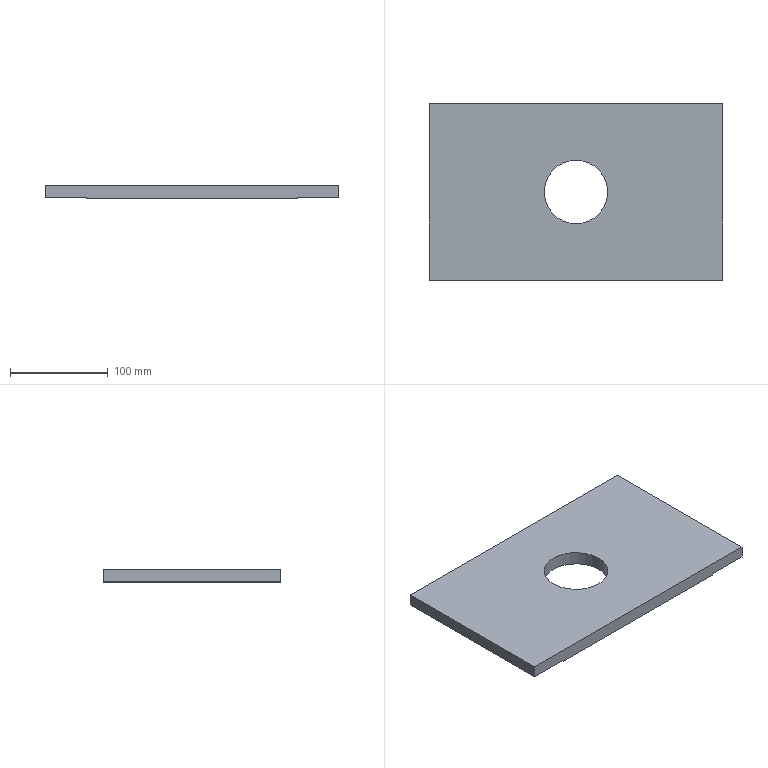Part | SolidWorks | features ICE 2, Extrusion 1 | 1 solid | 12 faces | box 300 x 180 x 14 mm | volume 686864 mm3 | plane 10 | cylinder 2 | commonest cylinder face diameters 65 x2
STEP:
#1=CARTESIAN_POINT('',(-32.5,0.,0.));
#2=VERTEX_POINT('',#1);
#3=CARTESIAN_POINT('',(32.5,0.,0.));
#4=VERTEX_POINT('',#3);
#5=CARTESIAN_POINT('',(0.,0.,0.));
#6=DIRECTION('',(0.,0.,1.));
#7=DIRECTION('',(-1.,0.,0.));
#8=AXIS2_PLACEMENT_3D('',#5,#6,#7);
#9=CIRCLE('',#8,32.5);
#10=EDGE_CURVE('',#2,#4,#9,.T.);
#11=ORIENTED_EDGE('',*,*,#10,.F.);
#12=CARTESIAN_POINT('',(-32.5,0.,14.));
#13=VERTEX_POINT('',#12);
#14=CARTESIAN_POINT('',(-32.5,0.,-0.001));
#15=DIRECTION('',(0.,0.,1.));
#16=VECTOR('',#15,1000.);
#17=LINE('',#14,#16);
#18=EDGE_CURVE('',#2,#13,#17,.T.);
#19=ORIENTED_EDGE('',*,*,#18,.T.);
#20=CARTESIAN_POINT('',(32.5,0.,14.));
#21=VERTEX_POINT('',#20);
#22=CARTESIAN_POINT('',(0.,0.,14.));
#23=DIRECTION('',(0.,0.,1.));
#24=DIRECTION('',(1.,0.,0.));
#25=AXIS2_PLACEMENT_3D('',#22,#23,#24);
#26=CIRCLE('',#25,32.5);
#27=EDGE_CURVE('',#13,#21,#26,.T.);
#28=ORIENTED_EDGE('',*,*,#27,.T.);
#29=CARTESIAN_POINT('',(32.5,0.,-0.001));
#30=DIRECTION('',(0.,0.,1.));
#31=VECTOR('',#30,1000.);
#32=LINE('',#29,#31);
#33=EDGE_CURVE('',#4,#21,#32,.T.);
#34=ORIENTED_EDGE('',*,*,#33,.F.);
#35=EDGE_LOOP('',(#11,#19,#28,#34));
#36=FACE_OUTER_BOUND('',#35,.T.);
#37=CARTESIAN_POINT('',(0.,0.,-0.001));
#38=DIRECTION('',(0.,0.,1.));
#39=DIRECTION('',(1.,0.,0.));
#40=AXIS2_PLACEMENT_3D('',#37,#38,#39);
#41=CYLINDRICAL_SURFACE('',#40,32.5);
#42=ADVANCED_FACE('',(#36),#41,.F.);
#43=CARTESIAN_POINT('',(-150.,-90.,1.5));
#44=VERTEX_POINT('',#43);
#45=CARTESIAN_POINT('',(-150.,90.,1.5));
#46=VERTEX_POINT('',#45);
#47=CARTESIAN_POINT('',(-150.,-90.,1.5));
#48=DIRECTION('',(0.,1.,0.));
#49=VECTOR('',#48,1000.);
#50=LINE('',#47,#49);
#51=EDGE_CURVE('',#44,#46,#50,.T.);
#52=ORIENTED_EDGE('',*,*,#51,.F.);
#53=CARTESIAN_POINT('',(-150.,-90.,14.));
#54=VERTEX_POINT('',#53);
#55=CARTESIAN_POINT('',(-150.,-90.,14.));
#56=DIRECTION('',(0.,0.,-1.));
#57=VECTOR('',#56,1000.);
#58=LINE('',#55,#57);
#59=EDGE_CURVE('',#54,#44,#58,.T.);
#60=ORIENTED_EDGE('',*,*,#59,.F.);
#61=CARTESIAN_POINT('',(-150.,90.,14.));
#62=VERTEX_POINT('',#61);
#63=CARTESIAN_POINT('',(-150.,-90.,14.));
#64=DIRECTION('',(0.,-1.,0.));
#65=VECTOR('',#64,1000.);
#66=LINE('',#63,#65);
#67=EDGE_CURVE('',#62,#54,#66,.T.);
#68=ORIENTED_EDGE('',*,*,#67,.F.);
#69=CARTESIAN_POINT('',(-150.,90.,14.));
#70=DIRECTION('',(0.,0.,-1.));
#71=VECTOR('',#70,1000.);
#72=LINE('',#69,#71);
#73=EDGE_CURVE('',#62,#46,#72,.T.);
#74=ORIENTED_EDGE('',*,*,#73,.T.);
#75=EDGE_LOOP('',(#52,#60,#68,#74));
#76=FACE_OUTER_BOUND('',#75,.T.);
#77=CARTESIAN_POINT('',(-150.,-90.,14.));
#78=DIRECTION('',(1.,0.,0.));
#79=DIRECTION('',(0.,0.,-1.));
#80=AXIS2_PLACEMENT_3D('',#77,#78,#79);
#81=PLANE('',#80);
#82=ADVANCED_FACE('',(#76),#81,.F.);
#83=CARTESIAN_POINT('',(150.,-90.,14.));
#84=VERTEX_POINT('',#83);
#85=CARTESIAN_POINT('',(150.,-90.,1.5));
#86=VERTEX_POINT('',#85);
#87=CARTESIAN_POINT('',(150.,-90.,14.));
#88=DIRECTION('',(0.,0.,-1.));
#89=VECTOR('',#88,1000.);
#90=LINE('',#87,#89);
#91=EDGE_CURVE('',#84,#86,#90,.T.);
#92=ORIENTED_EDGE('',*,*,#91,.T.);
#93=CARTESIAN_POINT('',(150.,90.,1.5));
#94=VERTEX_POINT('',#93);
#95=CARTESIAN_POINT('',(150.,-90.,1.5));
#96=DIRECTION('',(0.,-1.,0.));
#97=VECTOR('',#96,1000.);
#98=LINE('',#95,#97);
#99=EDGE_CURVE('',#94,#86,#98,.T.);
#100=ORIENTED_EDGE('',*,*,#99,.F.);
#101=CARTESIAN_POINT('',(150.,90.,14.));
#102=VERTEX_POINT('',#101);
#103=CARTESIAN_POINT('',(150.,90.,14.));
#104=DIRECTION('',(0.,0.,-1.));
#105=VECTOR('',#104,1000.);
#106=LINE('',#103,#105);
#107=EDGE_CURVE('',#102,#94,#106,.T.);
#108=ORIENTED_EDGE('',*,*,#107,.F.);
#109=CARTESIAN_POINT('',(150.,-90.,14.));
#110=DIRECTION('',(0.,1.,0.));
#111=VECTOR('',#110,1000.);
#112=LINE('',#109,#111);
#113=EDGE_CURVE('',#84,#102,#112,.T.);
#114=ORIENTED_EDGE('',*,*,#113,.F.);
#115=EDGE_LOOP('',(#92,#100,#108,#114));
#116=FACE_OUTER_BOUND('',#115,.T.);
#117=CARTESIAN_POINT('',(150.,-90.,14.));
#118=DIRECTION('',(-1.,0.,0.));
#119=DIRECTION('',(0.,0.,1.));
#120=AXIS2_PLACEMENT_3D('',#117,#118,#119);
#121=PLANE('',#120);
#122=ADVANCED_FACE('',(#116),#121,.F.);
#123=CARTESIAN_POINT('',(108.,90.,0.));
#124=VERTEX_POINT('',#123);
#125=CARTESIAN_POINT('',(-108.,90.,0.));
#126=VERTEX_POINT('',#125);
#127=CARTESIAN_POINT('',(-150.,90.,0.));
#128=DIRECTION('',(-1.,0.,0.));
#129=VECTOR('',#128,1000.);
#130=LINE('',#127,#129);
#131=EDGE_CURVE('',#124,#126,#130,.T.);
#132=ORIENTED_EDGE('',*,*,#131,.T.);
#133=CARTESIAN_POINT('',(-108.,90.,1.5));
#134=VERTEX_POINT('',#133);
#135=CARTESIAN_POINT('',(-108.,90.,1.5));
#136=DIRECTION('',(0.,0.,-1.));
#137=VECTOR('',#136,1000.);
#138=LINE('',#135,#137);
#139=EDGE_CURVE('',#134,#126,#138,.T.);
#140=ORIENTED_EDGE('',*,*,#139,.F.);
#141=CARTESIAN_POINT('',(-150.,90.,1.5));
#142=DIRECTION('',(1.,0.,0.));
#143=VECTOR('',#142,1000.);
#144=LINE('',#141,#143);
#145=EDGE_CURVE('',#46,#134,#144,.T.);
#146=ORIENTED_EDGE('',*,*,#145,.F.);
#147=ORIENTED_EDGE('',*,*,#73,.F.);
#148=CARTESIAN_POINT('',(-150.,90.,14.));
#149=DIRECTION('',(-1.,0.,0.));
#150=VECTOR('',#149,1000.);
#151=LINE('',#148,#150);
#152=EDGE_CURVE('',#102,#62,#151,.T.);
#153=ORIENTED_EDGE('',*,*,#152,.F.);
#154=ORIENTED_EDGE('',*,*,#107,.T.);
#155=CARTESIAN_POINT('',(108.,90.,1.5));
#156=VERTEX_POINT('',#155);
#157=CARTESIAN_POINT('',(150.,90.,1.5));
#158=DIRECTION('',(1.,0.,0.));
#159=VECTOR('',#158,1000.);
#160=LINE('',#157,#159);
#161=EDGE_CURVE('',#156,#94,#160,.T.);
#162=ORIENTED_EDGE('',*,*,#161,.F.);
#163=CARTESIAN_POINT('',(108.,90.,1.5));
#164=DIRECTION('',(0.,0.,-1.));
#165=VECTOR('',#164,1000.);
#166=LINE('',#163,#165);
#167=EDGE_CURVE('',#156,#124,#166,.T.);
#168=ORIENTED_EDGE('',*,*,#167,.T.);
#169=EDGE_LOOP('',(#132,#140,#146,#147,#153,#154,#162,#168));
#170=FACE_OUTER_BOUND('',#169,.T.);
#171=CARTESIAN_POINT('',(-150.,90.,14.));
#172=DIRECTION('',(0.,-1.,0.));
#173=DIRECTION('',(0.,0.,-1.));
#174=AXIS2_PLACEMENT_3D('',#171,#172,#173);
#175=PLANE('',#174);
#176=ADVANCED_FACE('',(#170),#175,.F.);
#177=CARTESIAN_POINT('',(-108.,-90.,1.5));
#178=VERTEX_POINT('',#177);
#179=CARTESIAN_POINT('',(-150.,-90.,1.5));
#180=DIRECTION('',(-1.,0.,0.));
#181=VECTOR('',#180,1000.);
#182=LINE('',#179,#181);
#183=EDGE_CURVE('',#178,#44,#182,.T.);
#184=ORIENTED_EDGE('',*,*,#183,.F.);
#185=CARTESIAN_POINT('',(-108.,-90.,0.));
#186=VERTEX_POINT('',#185);
#187=CARTESIAN_POINT('',(-108.,-90.,1.5));
#188=DIRECTION('',(0.,0.,-1.));
#189=VECTOR('',#188,1000.);
#190=LINE('',#187,#189);
#191=EDGE_CURVE('',#178,#186,#190,.T.);
#192=ORIENTED_EDGE('',*,*,#191,.T.);
#193=CARTESIAN_POINT('',(108.,-90.,0.));
#194=VERTEX_POINT('',#193);
#195=CARTESIAN_POINT('',(-150.,-90.,0.));
#196=DIRECTION('',(1.,0.,0.));
#197=VECTOR('',#196,1000.);
#198=LINE('',#195,#197);
#199=EDGE_CURVE('',#186,#194,#198,.T.);
#200=ORIENTED_EDGE('',*,*,#199,.T.);
#201=CARTESIAN_POINT('',(108.,-90.,1.5));
#202=VERTEX_POINT('',#201);
#203=CARTESIAN_POINT('',(108.,-90.,1.5));
#204=DIRECTION('',(0.,0.,-1.));
#205=VECTOR('',#204,1000.);
#206=LINE('',#203,#205);
#207=EDGE_CURVE('',#202,#194,#206,.T.);
#208=ORIENTED_EDGE('',*,*,#207,.F.);
#209=CARTESIAN_POINT('',(150.,-90.,1.5));
#210=DIRECTION('',(-1.,0.,0.));
#211=VECTOR('',#210,1000.);
#212=LINE('',#209,#211);
#213=EDGE_CURVE('',#86,#202,#212,.T.);
#214=ORIENTED_EDGE('',*,*,#213,.F.);
#215=ORIENTED_EDGE('',*,*,#91,.F.);
#216=CARTESIAN_POINT('',(-150.,-90.,14.));
#217=DIRECTION('',(1.,0.,0.));
#218=VECTOR('',#217,1000.);
#219=LINE('',#216,#218);
#220=EDGE_CURVE('',#54,#84,#219,.T.);
#221=ORIENTED_EDGE('',*,*,#220,.F.);
#222=ORIENTED_EDGE('',*,*,#59,.T.);
#223=EDGE_LOOP('',(#184,#192,#200,#208,#214,#215,#221,#222));
#224=FACE_OUTER_BOUND('',#223,.T.);
#225=CARTESIAN_POINT('',(-150.,-90.,14.));
#226=DIRECTION('',(0.,1.,0.));
#227=DIRECTION('',(0.,0.,1.));
#228=AXIS2_PLACEMENT_3D('',#225,#226,#227);
#229=PLANE('',#228);
#230=ADVANCED_FACE('',(#224),#229,.F.);
#231=CARTESIAN_POINT('',(0.,0.,14.));
#232=DIRECTION('',(0.,0.,1.));
#233=DIRECTION('',(1.,0.,0.));
#234=AXIS2_PLACEMENT_3D('',#231,#232,#233);
#235=CIRCLE('',#234,32.5);
#236=EDGE_CURVE('',#21,#13,#235,.T.);
#237=ORIENTED_EDGE('',*,*,#236,.F.);
#238=ORIENTED_EDGE('',*,*,#27,.F.);
#239=EDGE_LOOP('',(#237,#238));
#240=FACE_BOUND('',#239,.T.);
#241=ORIENTED_EDGE('',*,*,#113,.T.);
#242=ORIENTED_EDGE('',*,*,#152,.T.);
#243=ORIENTED_EDGE('',*,*,#67,.T.);
#244=ORIENTED_EDGE('',*,*,#220,.T.);
#245=EDGE_LOOP('',(#241,#242,#243,#244));
#246=FACE_OUTER_BOUND('',#245,.T.);
#247=CARTESIAN_POINT('',(0.,0.,14.));
#248=DIRECTION('',(0.,0.,-1.));
#249=DIRECTION('',(-1.,0.,0.));
#250=AXIS2_PLACEMENT_3D('',#247,#248,#249);
#251=PLANE('',#250);
#252=ADVANCED_FACE('',(#240,#246),#251,.F.);
#253=CARTESIAN_POINT('',(0.,0.,0.));
#254=DIRECTION('',(0.,0.,1.));
#255=DIRECTION('',(-1.,0.,0.));
#256=AXIS2_PLACEMENT_3D('',#253,#254,#255);
#257=CIRCLE('',#256,32.5);
#258=EDGE_CURVE('',#4,#2,#257,.T.);
#259=ORIENTED_EDGE('',*,*,#258,.T.);
#260=ORIENTED_EDGE('',*,*,#10,.T.);
#261=EDGE_LOOP('',(#259,#260));
#262=FACE_BOUND('',#261,.T.);
#263=CARTESIAN_POINT('',(-108.,-90.,0.));
#264=DIRECTION('',(0.,-1.,0.));
#265=VECTOR('',#264,1000.);
#266=LINE('',#263,#265);
#267=EDGE_CURVE('',#126,#186,#266,.T.);
#268=ORIENTED_EDGE('',*,*,#267,.F.);
#269=ORIENTED_EDGE('',*,*,#131,.F.);
#270=CARTESIAN_POINT('',(108.,-90.,0.));
#271=DIRECTION('',(0.,1.,0.));
#272=VECTOR('',#271,1000.);
#273=LINE('',#270,#272);
#274=EDGE_CURVE('',#194,#124,#273,.T.);
#275=ORIENTED_EDGE('',*,*,#274,.F.);
#276=ORIENTED_EDGE('',*,*,#199,.F.);
#277=EDGE_LOOP('',(#268,#269,#275,#276));
#278=FACE_OUTER_BOUND('',#277,.T.);
#279=CARTESIAN_POINT('',(0.,0.,0.));
#280=DIRECTION('',(0.,0.,-1.));
#281=DIRECTION('',(-1.,0.,0.));
#282=AXIS2_PLACEMENT_3D('',#279,#280,#281);
#283=PLANE('',#282);
#284=ADVANCED_FACE('',(#262,#278),#283,.T.);
#285=ORIENTED_EDGE('',*,*,#274,.T.);
#286=ORIENTED_EDGE('',*,*,#167,.F.);
#287=CARTESIAN_POINT('',(108.,-90.,1.5));
#288=DIRECTION('',(0.,1.,0.));
#289=VECTOR('',#288,1000.);
#290=LINE('',#287,#289);
#291=EDGE_CURVE('',#202,#156,#290,.T.);
#292=ORIENTED_EDGE('',*,*,#291,.F.);
#293=ORIENTED_EDGE('',*,*,#207,.T.);
#294=EDGE_LOOP('',(#285,#286,#292,#293));
#295=FACE_OUTER_BOUND('',#294,.T.);
#296=CARTESIAN_POINT('',(108.,-90.,1.5));
#297=DIRECTION('',(-1.,0.,0.));
#298=DIRECTION('',(0.,0.,1.));
#299=AXIS2_PLACEMENT_3D('',#296,#297,#298);
#300=PLANE('',#299);
#301=ADVANCED_FACE('',(#295),#300,.F.);
#302=ORIENTED_EDGE('',*,*,#99,.T.);
#303=ORIENTED_EDGE('',*,*,#213,.T.);
#304=ORIENTED_EDGE('',*,*,#291,.T.);
#305=ORIENTED_EDGE('',*,*,#161,.T.);
#306=EDGE_LOOP('',(#302,#303,#304,#305));
#307=FACE_OUTER_BOUND('',#306,.T.);
#308=CARTESIAN_POINT('',(0.,0.,1.5));
#309=DIRECTION('',(0.,0.,1.));
#310=DIRECTION('',(1.,0.,0.));
#311=AXIS2_PLACEMENT_3D('',#308,#309,#310);
#312=PLANE('',#311);
#313=ADVANCED_FACE('',(#307),#312,.F.);
#314=ORIENTED_EDGE('',*,*,#267,.T.);
#315=ORIENTED_EDGE('',*,*,#191,.F.);
#316=CARTESIAN_POINT('',(-108.,-90.,1.5));
#317=DIRECTION('',(0.,-1.,0.));
#318=VECTOR('',#317,1000.);
#319=LINE('',#316,#318);
#320=EDGE_CURVE('',#134,#178,#319,.T.);
#321=ORIENTED_EDGE('',*,*,#320,.F.);
#322=ORIENTED_EDGE('',*,*,#139,.T.);
#323=EDGE_LOOP('',(#314,#315,#321,#322));
#324=FACE_OUTER_BOUND('',#323,.T.);
#325=CARTESIAN_POINT('',(-108.,-90.,1.5));
#326=DIRECTION('',(1.,0.,0.));
#327=DIRECTION('',(0.,1.,0.));
#328=AXIS2_PLACEMENT_3D('',#325,#326,#327);
#329=PLANE('',#328);
#330=ADVANCED_FACE('',(#324),#329,.F.);
#331=ORIENTED_EDGE('',*,*,#51,.T.);
#332=ORIENTED_EDGE('',*,*,#145,.T.);
#333=ORIENTED_EDGE('',*,*,#320,.T.);
#334=ORIENTED_EDGE('',*,*,#183,.T.);
#335=EDGE_LOOP('',(#331,#332,#333,#334));
#336=FACE_OUTER_BOUND('',#335,.T.);
#337=CARTESIAN_POINT('',(0.,0.,1.5));
#338=DIRECTION('',(0.,0.,-1.));
#339=DIRECTION('',(-1.,0.,0.));
#340=AXIS2_PLACEMENT_3D('',#337,#338,#339);
#341=PLANE('',#340);
#342=ADVANCED_FACE('',(#336),#341,.T.);
#343=ORIENTED_EDGE('',*,*,#18,.F.);
#344=ORIENTED_EDGE('',*,*,#258,.F.);
#345=ORIENTED_EDGE('',*,*,#33,.T.);
#346=ORIENTED_EDGE('',*,*,#236,.T.);
#347=EDGE_LOOP('',(#343,#344,#345,#346));
#348=FACE_OUTER_BOUND('',#347,.T.);
#349=CARTESIAN_POINT('',(0.,0.,-0.001));
#350=DIRECTION('',(0.,0.,1.));
#351=DIRECTION('',(1.,0.,0.));
#352=AXIS2_PLACEMENT_3D('',#349,#350,#351);
#353=CYLINDRICAL_SURFACE('',#352,32.5);
#354=ADVANCED_FACE('',(#348),#353,.F.);
#355=CLOSED_SHELL('',(#42,#82,#122,#176,#230,#252,#284,#301,#313,#330,#342,#354));
#356=MANIFOLD_SOLID_BREP('',#355);
#357=CARTESIAN_POINT('',(0.,0.,0.));
#358=DIRECTION('',(0.,0.,1.));
#359=DIRECTION('',(1.,0.,0.));
#360=AXIS2_PLACEMENT_3D('',#357,#358,#359);
#361=(LENGTH_UNIT()NAMED_UNIT(*)SI_UNIT(.MILLI.,.METRE.));
#362=UNCERTAINTY_MEASURE_WITH_UNIT(LENGTH_MEASURE(0.00001),#361,'','');
#363=(NAMED_UNIT(*)PLANE_ANGLE_UNIT()SI_UNIT($,.RADIAN.));
#364=(NAMED_UNIT(*)SI_UNIT($,.STERADIAN.)SOLID_ANGLE_UNIT());
#365=(GEOMETRIC_REPRESENTATION_CONTEXT(3)GLOBAL_UNCERTAINTY_ASSIGNED_CONTEXT((#362))GLOBAL_UNIT_ASSIGNED_CONTEXT((#361,#363,#364))REPRESENTATION_CONTEXT('',''));
#366=ADVANCED_BREP_SHAPE_REPRESENTATION('',(#356,#360),#365);